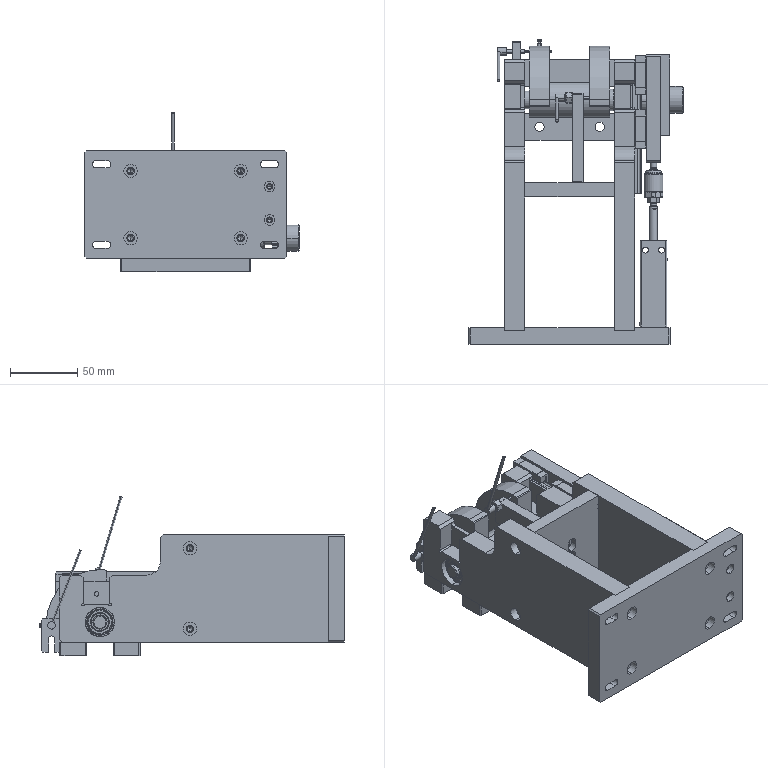Part | SolidWorks | 31 solids | 2035 faces | box 159.5 x 226.8 x 118.648 mm | volume 777455 mm3 | plane 857 | cylinder 681 | cone 256 | spline 241 | commonest cylinder face diameters 0.5 x62 3 x41 0.4 x40 10 x36 6 x30 4.5 x29